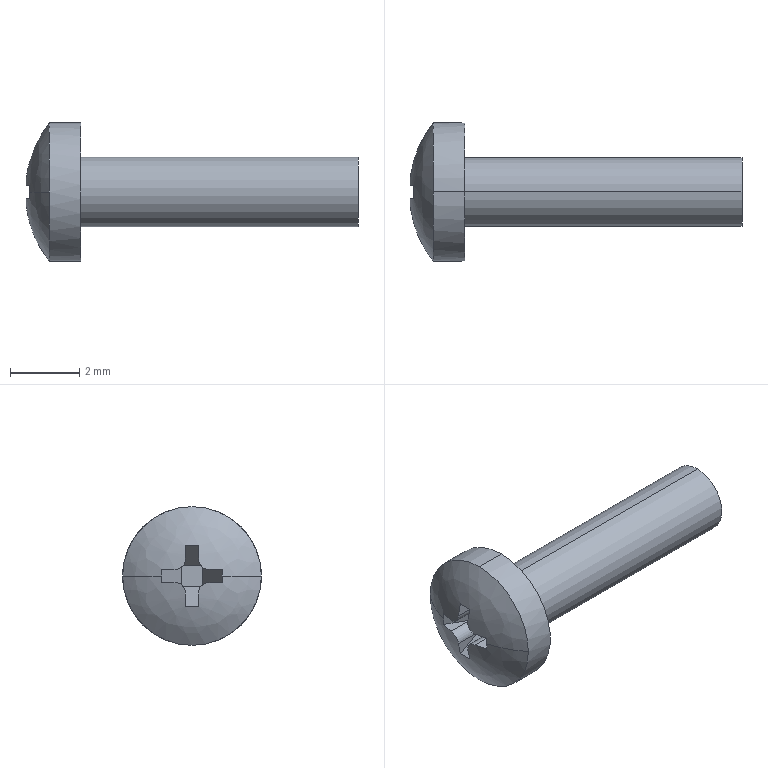Part | SolidWorks | features BaseBody 1 | 1 solid | 25 faces | box 9.576 x 4 x 4 mm | volume 40.085 mm3 | plane 15 | cylinder 8 | spline 2 | commonest cylinder face diameters 0.6 x4 2 x2 4 x2
STEP:
#1=CARTESIAN_POINT('',(0.702,2.,0.));
#2=VERTEX_POINT('',#1);
#3=CARTESIAN_POINT('',(0.702,0.,2.));
#4=VERTEX_POINT('',#3);
#5=CARTESIAN_POINT('',(0.702,0.,0.));
#6=DIRECTION('',(1.,0.,0.));
#7=DIRECTION('',(0.,0.,-1.));
#8=AXIS2_PLACEMENT_3D('',#5,#6,#7);
#9=CIRCLE('',#8,2.);
#10=EDGE_CURVE('',#2,#4,#9,.T.);
#11=ORIENTED_EDGE('',*,*,#10,.F.);
#12=CARTESIAN_POINT('',(0.1231,0.8789,0.));
#13=VERTEX_POINT('',#12);
#14=CARTESIAN_POINT('',(3.2,0.,0.));
#15=DIRECTION('',(0.,0.,1.));
#16=DIRECTION('',(0.,1.,0.));
#17=AXIS2_PLACEMENT_3D('',#14,#15,#16);
#18=CIRCLE('',#17,3.2);
#19=EDGE_CURVE('',#2,#13,#18,.T.);
#20=ORIENTED_EDGE('',*,*,#19,.T.);
#21=CARTESIAN_POINT('',(0.1281,0.876,0.19));
#22=VERTEX_POINT('',#21);
#23=CARTESIAN_POINT('',(0.1231,0.8789,0.));
#24=CARTESIAN_POINT('',(0.1231,0.8789,0.06339));
#25=CARTESIAN_POINT('',(0.1248,0.878,0.1267));
#26=CARTESIAN_POINT('',(0.1281,0.876,0.19));
#27=B_SPLINE_CURVE_WITH_KNOTS('',3,(#23,#24,#25,#26),.UNSPECIFIED.,.F.,.F.,(4,4),(0.,1.),.UNSPECIFIED.);
#28=EDGE_CURVE('',#13,#22,#27,.T.);
#29=ORIENTED_EDGE('',*,*,#28,.T.);
#30=CARTESIAN_POINT('',(0.04345,0.49,0.19));
#31=VERTEX_POINT('',#30);
#32=CARTESIAN_POINT('',(0.1281,0.876,0.19));
#33=CARTESIAN_POINT('',(0.09192,0.7491,0.19));
#34=CARTESIAN_POINT('',(0.0637,0.6204,0.19));
#35=CARTESIAN_POINT('',(0.04345,0.49,0.19));
#36=B_SPLINE_CURVE_WITH_KNOTS('',3,(#32,#33,#34,#35),.UNSPECIFIED.,.F.,.F.,(4,4),(0.,0.0003952),.UNSPECIFIED.);
#37=EDGE_CURVE('',#22,#31,#36,.T.);
#38=ORIENTED_EDGE('',*,*,#37,.T.);
#39=CARTESIAN_POINT('',(0.04345,0.19,0.49));
#40=VERTEX_POINT('',#39);
#41=CARTESIAN_POINT('',(0.04345,0.49,0.19));
#42=CARTESIAN_POINT('',(0.03125,0.4114,0.19));
#43=CARTESIAN_POINT('',(0.02423,0.3335,0.2223));
#44=CARTESIAN_POINT('',(0.02421,0.2224,0.3333));
#45=CARTESIAN_POINT('',(0.03125,0.19,0.4114));
#46=CARTESIAN_POINT('',(0.04345,0.19,0.49));
#47=B_SPLINE_CURVE_WITH_KNOTS('',3,(#41,#42,#43,#44,#45,#46),.UNSPECIFIED.,.F.,.F.,(4,2,4),(0.,0.0002354,0.0004707),.UNSPECIFIED.);
#48=EDGE_CURVE('',#31,#40,#47,.T.);
#49=ORIENTED_EDGE('',*,*,#48,.T.);
#50=CARTESIAN_POINT('',(0.1281,0.19,0.876));
#51=VERTEX_POINT('',#50);
#52=CARTESIAN_POINT('',(3.2,0.19,0.));
#53=DIRECTION('',(0.,1.,0.));
#54=DIRECTION('',(0.,0.,1.));
#55=AXIS2_PLACEMENT_3D('',#52,#53,#54);
#56=CIRCLE('',#55,3.194);
#57=EDGE_CURVE('',#40,#51,#56,.T.);
#58=ORIENTED_EDGE('',*,*,#57,.T.);
#59=CARTESIAN_POINT('',(0.1281,-0.19,0.876));
#60=VERTEX_POINT('',#59);
#61=CARTESIAN_POINT('',(0.1281,0.19,0.876));
#62=CARTESIAN_POINT('',(0.1214,0.06333,0.8799));
#63=CARTESIAN_POINT('',(0.1214,-0.06333,0.8799));
#64=CARTESIAN_POINT('',(0.1281,-0.19,0.876));
#65=B_SPLINE_CURVE_WITH_KNOTS('',3,(#61,#62,#63,#64),.UNSPECIFIED.,.F.,.F.,(4,4),(0.,0.00038),.UNSPECIFIED.);
#66=EDGE_CURVE('',#51,#60,#65,.T.);
#67=ORIENTED_EDGE('',*,*,#66,.T.);
#68=CARTESIAN_POINT('',(0.04345,-0.19,0.49));
#69=VERTEX_POINT('',#68);
#70=CARTESIAN_POINT('',(3.2,-0.19,0.));
#71=DIRECTION('',(0.,-1.,0.));
#72=DIRECTION('',(0.,0.,1.));
#73=AXIS2_PLACEMENT_3D('',#70,#71,#72);
#74=CIRCLE('',#73,3.194);
#75=EDGE_CURVE('',#60,#69,#74,.T.);
#76=ORIENTED_EDGE('',*,*,#75,.T.);
#77=CARTESIAN_POINT('',(0.04345,-0.49,0.19));
#78=VERTEX_POINT('',#77);
#79=CARTESIAN_POINT('',(0.04345,-0.19,0.49));
#80=CARTESIAN_POINT('',(0.03125,-0.19,0.4114));
#81=CARTESIAN_POINT('',(0.02423,-0.2223,0.3335));
#82=CARTESIAN_POINT('',(0.02421,-0.3333,0.2224));
#83=CARTESIAN_POINT('',(0.03125,-0.4114,0.19));
#84=CARTESIAN_POINT('',(0.04345,-0.49,0.19));
#85=B_SPLINE_CURVE_WITH_KNOTS('',3,(#79,#80,#81,#82,#83,#84),.UNSPECIFIED.,.F.,.F.,(4,2,4),(0.,0.0002354,0.0004707),.UNSPECIFIED.);
#86=EDGE_CURVE('',#69,#78,#85,.T.);
#87=ORIENTED_EDGE('',*,*,#86,.T.);
#88=CARTESIAN_POINT('',(0.1281,-0.876,0.19));
#89=VERTEX_POINT('',#88);
#90=CARTESIAN_POINT('',(0.04345,-0.49,0.19));
#91=CARTESIAN_POINT('',(0.0637,-0.6204,0.19));
#92=CARTESIAN_POINT('',(0.09192,-0.7491,0.19));
#93=CARTESIAN_POINT('',(0.1281,-0.876,0.19));
#94=B_SPLINE_CURVE_WITH_KNOTS('',3,(#90,#91,#92,#93),.UNSPECIFIED.,.F.,.F.,(4,4),(0.,0.0003952),.UNSPECIFIED.);
#95=EDGE_CURVE('',#78,#89,#94,.T.);
#96=ORIENTED_EDGE('',*,*,#95,.T.);
#97=CARTESIAN_POINT('',(0.1231,-0.8789,0.));
#98=VERTEX_POINT('',#97);
#99=CARTESIAN_POINT('',(0.1281,-0.876,0.19));
#100=CARTESIAN_POINT('',(0.1248,-0.878,0.1267));
#101=CARTESIAN_POINT('',(0.1231,-0.8789,0.06339));
#102=CARTESIAN_POINT('',(0.1231,-0.8789,0.));
#103=B_SPLINE_CURVE_WITH_KNOTS('',3,(#99,#100,#101,#102),.UNSPECIFIED.,.F.,.F.,(4,4),(0.,1.),.UNSPECIFIED.);
#104=EDGE_CURVE('',#89,#98,#103,.T.);
#105=ORIENTED_EDGE('',*,*,#104,.T.);
#106=CARTESIAN_POINT('',(0.702,-2.,0.));
#107=VERTEX_POINT('',#106);
#108=CARTESIAN_POINT('',(3.2,0.,0.));
#109=DIRECTION('',(0.,0.,1.));
#110=DIRECTION('',(0.,1.,0.));
#111=AXIS2_PLACEMENT_3D('',#108,#109,#110);
#112=CIRCLE('',#111,3.2);
#113=EDGE_CURVE('',#98,#107,#112,.T.);
#114=ORIENTED_EDGE('',*,*,#113,.T.);
#115=CARTESIAN_POINT('',(0.702,0.,0.));
#116=DIRECTION('',(1.,0.,0.));
#117=DIRECTION('',(0.,0.,-1.));
#118=AXIS2_PLACEMENT_3D('',#115,#116,#117);
#119=CIRCLE('',#118,2.);
#120=EDGE_CURVE('',#4,#107,#119,.T.);
#121=ORIENTED_EDGE('',*,*,#120,.F.);
#122=EDGE_LOOP('',(#11,#20,#29,#38,#49,#58,#67,#76,#87,#96,#105,#114,#121));
#123=FACE_OUTER_BOUND('',#122,.T.);
#124=CARTESIAN_POINT('',(0.7183,2.02,0.));
#125=CARTESIAN_POINT('',(0.7183,2.02,0.5729));
#126=CARTESIAN_POINT('',(0.9091,2.02,1.113));
#127=CARTESIAN_POINT('',(1.269,2.02,1.559));
#128=CARTESIAN_POINT('',(-0.2816,0.7919,0.));
#129=CARTESIAN_POINT('',(-0.2816,0.7919,0.8037));
#130=CARTESIAN_POINT('',(-0.01383,0.7919,1.562));
#131=CARTESIAN_POINT('',(0.491,0.7919,2.187));
#132=CARTESIAN_POINT('',(-0.2816,-0.7919,0.));
#133=CARTESIAN_POINT('',(-0.2816,-0.7919,0.8037));
#134=CARTESIAN_POINT('',(-0.01383,-0.7919,1.562));
#135=CARTESIAN_POINT('',(0.491,-0.7919,2.187));
#136=CARTESIAN_POINT('',(0.7183,-2.02,0.));
#137=CARTESIAN_POINT('',(0.7183,-2.02,0.5729));
#138=CARTESIAN_POINT('',(0.9091,-2.02,1.113));
#139=CARTESIAN_POINT('',(1.269,-2.02,1.559));
#140=(BOUNDED_SURFACE()B_SPLINE_SURFACE(3,3,((#124,#125,#126,#127),(#128,#129,#130,#131),(#132,#133,#134,#135),(#136,#137,#138,#139)),.UNSPECIFIED.,.F.,.F.,.F.)B_SPLINE_SURFACE_WITH_KNOTS((4,4),(4,4),(0.,1.),(0.,1.),.UNSPECIFIED.)GEOMETRIC_REPRESENTATION_ITEM()RATIONAL_B_SPLINE_SURFACE(((1.,0.9619,0.9619,1.),(0.8504,0.818,0.818,0.8504),(0.8504,0.818,0.818,0.8504),(1.,0.9619,0.9619,1.)))REPRESENTATION_ITEM('')SURFACE());
#141=ADVANCED_FACE('',(#123),#140,.T.);
#142=CARTESIAN_POINT('',(1.6,0.,-1.));
#143=VERTEX_POINT('',#142);
#144=CARTESIAN_POINT('',(1.6,0.,1.));
#145=VERTEX_POINT('',#144);
#146=CARTESIAN_POINT('',(1.6,0.,0.));
#147=DIRECTION('',(1.,0.,0.));
#148=DIRECTION('',(0.,0.,-1.));
#149=AXIS2_PLACEMENT_3D('',#146,#147,#148);
#150=CIRCLE('',#149,1.);
#151=EDGE_CURVE('',#143,#145,#150,.T.);
#152=ORIENTED_EDGE('',*,*,#151,.T.);
#153=CARTESIAN_POINT('',(9.6,0.,1.));
#154=VERTEX_POINT('',#153);
#155=CARTESIAN_POINT('',(4.516,0.,1.));
#156=DIRECTION('',(1.,0.,0.));
#157=VECTOR('',#156,1000.);
#158=LINE('',#155,#157);
#159=EDGE_CURVE('',#145,#154,#158,.T.);
#160=ORIENTED_EDGE('',*,*,#159,.T.);
#161=CARTESIAN_POINT('',(9.6,0.,-1.));
#162=VERTEX_POINT('',#161);
#163=CARTESIAN_POINT('',(9.6,0.,0.));
#164=DIRECTION('',(-1.,0.,0.));
#165=DIRECTION('',(0.,0.,-1.));
#166=AXIS2_PLACEMENT_3D('',#163,#164,#165);
#167=CIRCLE('',#166,1.);
#168=EDGE_CURVE('',#154,#162,#167,.T.);
#169=ORIENTED_EDGE('',*,*,#168,.T.);
#170=CARTESIAN_POINT('',(4.516,0.,-1.));
#171=DIRECTION('',(1.,0.,0.));
#172=VECTOR('',#171,1000.);
#173=LINE('',#170,#172);
#174=EDGE_CURVE('',#143,#162,#173,.T.);
#175=ORIENTED_EDGE('',*,*,#174,.F.);
#176=EDGE_LOOP('',(#152,#160,#169,#175));
#177=FACE_OUTER_BOUND('',#176,.T.);
#178=CARTESIAN_POINT('',(4.516,0.,0.));
#179=DIRECTION('',(1.,0.,0.));
#180=DIRECTION('',(0.,0.,-1.));
#181=AXIS2_PLACEMENT_3D('',#178,#179,#180);
#182=CYLINDRICAL_SURFACE('',#181,1.);
#183=ADVANCED_FACE('',(#177),#182,.T.);
#184=CARTESIAN_POINT('',(0.702,0.,-2.));
#185=VERTEX_POINT('',#184);
#186=CARTESIAN_POINT('',(0.702,0.,0.));
#187=DIRECTION('',(1.,0.,0.));
#188=DIRECTION('',(0.,0.,-1.));
#189=AXIS2_PLACEMENT_3D('',#186,#187,#188);
#190=CIRCLE('',#189,2.);
#191=EDGE_CURVE('',#185,#2,#190,.T.);
#192=ORIENTED_EDGE('',*,*,#191,.T.);
#193=ORIENTED_EDGE('',*,*,#10,.T.);
#194=CARTESIAN_POINT('',(1.6,0.,2.));
#195=VERTEX_POINT('',#194);
#196=CARTESIAN_POINT('',(4.516,0.,2.));
#197=DIRECTION('',(1.,0.,0.));
#198=VECTOR('',#197,1000.);
#199=LINE('',#196,#198);
#200=EDGE_CURVE('',#4,#195,#199,.T.);
#201=ORIENTED_EDGE('',*,*,#200,.T.);
#202=CARTESIAN_POINT('',(1.6,0.,-2.));
#203=VERTEX_POINT('',#202);
#204=CARTESIAN_POINT('',(1.6,0.,0.));
#205=DIRECTION('',(1.,0.,0.));
#206=DIRECTION('',(0.,0.,-1.));
#207=AXIS2_PLACEMENT_3D('',#204,#205,#206);
#208=CIRCLE('',#207,2.);
#209=EDGE_CURVE('',#203,#195,#208,.T.);
#210=ORIENTED_EDGE('',*,*,#209,.F.);
#211=CARTESIAN_POINT('',(4.516,0.,-2.));
#212=DIRECTION('',(1.,0.,0.));
#213=VECTOR('',#212,1000.);
#214=LINE('',#211,#213);
#215=EDGE_CURVE('',#185,#203,#214,.T.);
#216=ORIENTED_EDGE('',*,*,#215,.F.);
#217=EDGE_LOOP('',(#192,#193,#201,#210,#216));
#218=FACE_OUTER_BOUND('',#217,.T.);
#219=CARTESIAN_POINT('',(4.516,0.,0.));
#220=DIRECTION('',(1.,0.,0.));
#221=DIRECTION('',(0.,0.,-1.));
#222=AXIS2_PLACEMENT_3D('',#219,#220,#221);
#223=CYLINDRICAL_SURFACE('',#222,2.);
#224=ADVANCED_FACE('',(#218),#223,.T.);
#225=ORIENTED_EDGE('',*,*,#159,.F.);
#226=CARTESIAN_POINT('',(1.6,0.,0.));
#227=DIRECTION('',(1.,0.,0.));
#228=DIRECTION('',(0.,0.,-1.));
#229=AXIS2_PLACEMENT_3D('',#226,#227,#228);
#230=CIRCLE('',#229,1.);
#231=EDGE_CURVE('',#145,#143,#230,.T.);
#232=ORIENTED_EDGE('',*,*,#231,.T.);
#233=ORIENTED_EDGE('',*,*,#174,.T.);
#234=CARTESIAN_POINT('',(9.6,0.,0.));
#235=DIRECTION('',(-1.,0.,0.));
#236=DIRECTION('',(0.,0.,-1.));
#237=AXIS2_PLACEMENT_3D('',#234,#235,#236);
#238=CIRCLE('',#237,1.);
#239=EDGE_CURVE('',#162,#154,#238,.T.);
#240=ORIENTED_EDGE('',*,*,#239,.T.);
#241=EDGE_LOOP('',(#225,#232,#233,#240));
#242=FACE_OUTER_BOUND('',#241,.T.);
#243=CARTESIAN_POINT('',(4.516,0.,0.));
#244=DIRECTION('',(1.,0.,0.));
#245=DIRECTION('',(0.,0.,-1.));
#246=AXIS2_PLACEMENT_3D('',#243,#244,#245);
#247=CYLINDRICAL_SURFACE('',#246,1.);
#248=ADVANCED_FACE('',(#242),#247,.T.);
#249=ORIENTED_EDGE('',*,*,#239,.F.);
#250=ORIENTED_EDGE('',*,*,#168,.F.);
#251=EDGE_LOOP('',(#249,#250));
#252=FACE_OUTER_BOUND('',#251,.T.);
#253=CARTESIAN_POINT('',(9.6,1.,0.));
#254=DIRECTION('',(1.,0.,0.));
#255=DIRECTION('',(0.,0.,-1.));
#256=AXIS2_PLACEMENT_3D('',#253,#254,#255);
#257=PLANE('',#256);
#258=ADVANCED_FACE('',(#252),#257,.T.);
#259=ORIENTED_EDGE('',*,*,#151,.F.);
#260=ORIENTED_EDGE('',*,*,#231,.F.);
#261=EDGE_LOOP('',(#259,#260));
#262=FACE_BOUND('',#261,.T.);
#263=ORIENTED_EDGE('',*,*,#209,.T.);
#264=CARTESIAN_POINT('',(1.6,0.,0.));
#265=DIRECTION('',(1.,0.,0.));
#266=DIRECTION('',(0.,0.,-1.));
#267=AXIS2_PLACEMENT_3D('',#264,#265,#266);
#268=CIRCLE('',#267,2.);
#269=EDGE_CURVE('',#195,#203,#268,.T.);
#270=ORIENTED_EDGE('',*,*,#269,.T.);
#271=EDGE_LOOP('',(#263,#270));
#272=FACE_OUTER_BOUND('',#271,.T.);
#273=CARTESIAN_POINT('',(1.6,1.3,0.));
#274=DIRECTION('',(1.,0.,0.));
#275=DIRECTION('',(0.,0.,-1.));
#276=AXIS2_PLACEMENT_3D('',#273,#274,#275);
#277=PLANE('',#276);
#278=ADVANCED_FACE('',(#262,#272),#277,.T.);
#279=ORIENTED_EDGE('',*,*,#200,.F.);
#280=ORIENTED_EDGE('',*,*,#120,.T.);
#281=CARTESIAN_POINT('',(0.702,0.,0.));
#282=DIRECTION('',(1.,0.,0.));
#283=DIRECTION('',(0.,0.,-1.));
#284=AXIS2_PLACEMENT_3D('',#281,#282,#283);
#285=CIRCLE('',#284,2.);
#286=EDGE_CURVE('',#107,#185,#285,.T.);
#287=ORIENTED_EDGE('',*,*,#286,.T.);
#288=ORIENTED_EDGE('',*,*,#215,.T.);
#289=ORIENTED_EDGE('',*,*,#269,.F.);
#290=EDGE_LOOP('',(#279,#280,#287,#288,#289));
#291=FACE_OUTER_BOUND('',#290,.T.);
#292=CARTESIAN_POINT('',(4.516,0.,0.));
#293=DIRECTION('',(1.,0.,0.));
#294=DIRECTION('',(0.,0.,-1.));
#295=AXIS2_PLACEMENT_3D('',#292,#293,#294);
#296=CYLINDRICAL_SURFACE('',#295,2.);
#297=ADVANCED_FACE('',(#291),#296,.T.);
#298=ORIENTED_EDGE('',*,*,#19,.F.);
#299=ORIENTED_EDGE('',*,*,#191,.F.);
#300=ORIENTED_EDGE('',*,*,#286,.F.);
#301=ORIENTED_EDGE('',*,*,#113,.F.);
#302=CARTESIAN_POINT('',(0.1281,-0.876,-0.19));
#303=VERTEX_POINT('',#302);
#304=CARTESIAN_POINT('',(0.1231,-0.8789,0.));
#305=CARTESIAN_POINT('',(0.1231,-0.8789,-0.06339));
#306=CARTESIAN_POINT('',(0.1248,-0.878,-0.1267));
#307=CARTESIAN_POINT('',(0.1281,-0.876,-0.19));
#308=B_SPLINE_CURVE_WITH_KNOTS('',3,(#304,#305,#306,#307),.UNSPECIFIED.,.F.,.F.,(4,4),(0.,1.),.UNSPECIFIED.);
#309=EDGE_CURVE('',#98,#303,#308,.T.);
#310=ORIENTED_EDGE('',*,*,#309,.T.);
#311=CARTESIAN_POINT('',(0.04345,-0.49,-0.19));
#312=VERTEX_POINT('',#311);
#313=CARTESIAN_POINT('',(0.1281,-0.876,-0.19));
#314=CARTESIAN_POINT('',(0.09192,-0.7491,-0.19));
#315=CARTESIAN_POINT('',(0.0637,-0.6204,-0.19));
#316=CARTESIAN_POINT('',(0.04345,-0.49,-0.19));
#317=B_SPLINE_CURVE_WITH_KNOTS('',3,(#313,#314,#315,#316),.UNSPECIFIED.,.F.,.F.,(4,4),(0.,0.0003952),.UNSPECIFIED.);
#318=EDGE_CURVE('',#303,#312,#317,.T.);
#319=ORIENTED_EDGE('',*,*,#318,.T.);
#320=CARTESIAN_POINT('',(0.04345,-0.19,-0.49));
#321=VERTEX_POINT('',#320);
#322=CARTESIAN_POINT('',(0.04345,-0.49,-0.19));
#323=CARTESIAN_POINT('',(0.03125,-0.4114,-0.19));
#324=CARTESIAN_POINT('',(0.02423,-0.3335,-0.2223));
#325=CARTESIAN_POINT('',(0.02421,-0.2224,-0.3333));
#326=CARTESIAN_POINT('',(0.03125,-0.19,-0.4114));
#327=CARTESIAN_POINT('',(0.04345,-0.19,-0.49));
#328=B_SPLINE_CURVE_WITH_KNOTS('',3,(#322,#323,#324,#325,#326,#327),.UNSPECIFIED.,.F.,.F.,(4,2,4),(0.,0.0002354,0.0004707),.UNSPECIFIED.);
#329=EDGE_CURVE('',#312,#321,#328,.T.);
#330=ORIENTED_EDGE('',*,*,#329,.T.);
#331=CARTESIAN_POINT('',(0.1281,-0.19,-0.876));
#332=VERTEX_POINT('',#331);
#333=CARTESIAN_POINT('',(3.2,-0.19,0.));
#334=DIRECTION('',(0.,-1.,0.));
#335=DIRECTION('',(0.,0.,1.));
#336=AXIS2_PLACEMENT_3D('',#333,#334,#335);
#337=CIRCLE('',#336,3.194);
#338=EDGE_CURVE('',#321,#332,#337,.T.);
#339=ORIENTED_EDGE('',*,*,#338,.T.);
#340=CARTESIAN_POINT('',(0.1281,0.19,-0.876));
#341=VERTEX_POINT('',#340);
#342=CARTESIAN_POINT('',(0.1281,-0.19,-0.876));
#343=CARTESIAN_POINT('',(0.1214,-0.06333,-0.8799));
#344=CARTESIAN_POINT('',(0.1214,0.06333,-0.8799));
#345=CARTESIAN_POINT('',(0.1281,0.19,-0.876));
#346=B_SPLINE_CURVE_WITH_KNOTS('',3,(#342,#343,#344,#345),.UNSPECIFIED.,.F.,.F.,(4,4),(0.,0.00038),.UNSPECIFIED.);
#347=EDGE_CURVE('',#332,#341,#346,.T.);
#348=ORIENTED_EDGE('',*,*,#347,.T.);
#349=CARTESIAN_POINT('',(0.04345,0.19,-0.49));
#350=VERTEX_POINT('',#349);
#351=CARTESIAN_POINT('',(3.2,0.19,0.));
#352=DIRECTION('',(0.,1.,0.));
#353=DIRECTION('',(0.,0.,1.));
#354=AXIS2_PLACEMENT_3D('',#351,#352,#353);
#355=CIRCLE('',#354,3.194);
#356=EDGE_CURVE('',#341,#350,#355,.T.);
#357=ORIENTED_EDGE('',*,*,#356,.T.);
#358=CARTESIAN_POINT('',(0.04345,0.49,-0.19));
#359=VERTEX_POINT('',#358);
#360=CARTESIAN_POINT('',(0.04345,0.19,-0.49));
#361=CARTESIAN_POINT('',(0.03125,0.19,-0.4114));
#362=CARTESIAN_POINT('',(0.02423,0.2223,-0.3335));
#363=CARTESIAN_POINT('',(0.02421,0.3333,-0.2224));
#364=CARTESIAN_POINT('',(0.03125,0.4114,-0.19));
#365=CARTESIAN_POINT('',(0.04345,0.49,-0.19));
#366=B_SPLINE_CURVE_WITH_KNOTS('',3,(#360,#361,#362,#363,#364,#365),.UNSPECIFIED.,.F.,.F.,(4,2,4),(0.,0.0002354,0.0004707),.UNSPECIFIED.);
#367=EDGE_CURVE('',#350,#359,#366,.T.);
#368=ORIENTED_EDGE('',*,*,#367,.T.);
#369=CARTESIAN_POINT('',(0.1281,0.876,-0.19));
#370=VERTEX_POINT('',#369);
#371=CARTESIAN_POINT('',(0.04345,0.49,-0.19));
#372=CARTESIAN_POINT('',(0.0637,0.6204,-0.19));
#373=CARTESIAN_POINT('',(0.09192,0.7491,-0.19));
#374=CARTESIAN_POINT('',(0.1281,0.876,-0.19));
#375=B_SPLINE_CURVE_WITH_KNOTS('',3,(#371,#372,#373,#374),.UNSPECIFIED.,.F.,.F.,(4,4),(0.,0.0003952),.UNSPECIFIED.);
#376=EDGE_CURVE('',#359,#370,#375,.T.);
#377=ORIENTED_EDGE('',*,*,#376,.T.);
#378=CARTESIAN_POINT('',(0.1281,0.876,-0.19));
#379=CARTESIAN_POINT('',(0.1248,0.878,-0.1267));
#380=CARTESIAN_POINT('',(0.1231,0.8789,-0.06339));
#381=CARTESIAN_POINT('',(0.1231,0.8789,0.));
#382=B_SPLINE_CURVE_WITH_KNOTS('',3,(#378,#379,#380,#381),.UNSPECIFIED.,.F.,.F.,(4,4),(0.,1.),.UNSPECIFIED.);
#383=EDGE_CURVE('',#370,#13,#382,.T.);
#384=ORIENTED_EDGE('',*,*,#383,.T.);
#385=EDGE_LOOP('',(#298,#299,#300,#301,#310,#319,#330,#339,#348,#357,#368,#377,#384));
#386=FACE_OUTER_BOUND('',#385,.T.);
#387=CARTESIAN_POINT('',(1.269,2.02,-1.559));
#388=CARTESIAN_POINT('',(0.9091,2.02,-1.113));
#389=CARTESIAN_POINT('',(0.7183,2.02,-0.5729));
#390=CARTESIAN_POINT('',(0.7183,2.02,0.));
#391=CARTESIAN_POINT('',(0.491,0.7919,-2.187));
#392=CARTESIAN_POINT('',(-0.01383,0.7919,-1.562));
#393=CARTESIAN_POINT('',(-0.2816,0.7919,-0.8037));
#394=CARTESIAN_POINT('',(-0.2816,0.7919,0.));
#395=CARTESIAN_POINT('',(0.491,-0.7919,-2.187));
#396=CARTESIAN_POINT('',(-0.01383,-0.7919,-1.562));
#397=CARTESIAN_POINT('',(-0.2816,-0.7919,-0.8037));
#398=CARTESIAN_POINT('',(-0.2816,-0.7919,0.));
#399=CARTESIAN_POINT('',(1.269,-2.02,-1.559));
#400=CARTESIAN_POINT('',(0.9091,-2.02,-1.113));
#401=CARTESIAN_POINT('',(0.7183,-2.02,-0.5729));
#402=CARTESIAN_POINT('',(0.7183,-2.02,0.));
#403=(BOUNDED_SURFACE()B_SPLINE_SURFACE(3,3,((#387,#388,#389,#390),(#391,#392,#393,#394),(#395,#396,#397,#398),(#399,#400,#401,#402)),.UNSPECIFIED.,.F.,.F.,.F.)B_SPLINE_SURFACE_WITH_KNOTS((4,4),(4,4),(0.,1.),(0.,1.),.UNSPECIFIED.)GEOMETRIC_REPRESENTATION_ITEM()RATIONAL_B_SPLINE_SURFACE(((1.,0.9619,0.9619,1.),(0.8504,0.818,0.818,0.8504),(0.8504,0.818,0.818,0.8504),(1.,0.9619,0.9619,1.)))REPRESENTATION_ITEM('')SURFACE());
#404=ADVANCED_FACE('',(#386),#403,.T.);
#405=ORIENTED_EDGE('',*,*,#28,.F.);
#406=ORIENTED_EDGE('',*,*,#383,.F.);
#407=CARTESIAN_POINT('',(0.7967,0.49,-0.19));
#408=VERTEX_POINT('',#407);
#409=CARTESIAN_POINT('',(0.,0.95,-0.19));
#410=DIRECTION('',(0.866,-0.5,0.));
#411=VECTOR('',#410,1000.);
#412=LINE('',#409,#411);
#413=EDGE_CURVE('',#370,#408,#412,.T.);
#414=ORIENTED_EDGE('',*,*,#413,.T.);
#415=CARTESIAN_POINT('',(1.12,0.3034,-0.2551));
#416=VERTEX_POINT('',#415);
#417=CARTESIAN_POINT('',(0.7967,0.49,-0.19));
#418=CARTESIAN_POINT('',(0.9153,0.4216,-0.19));
#419=CARTESIAN_POINT('',(1.027,0.3569,-0.2125));
#420=CARTESIAN_POINT('',(1.12,0.3034,-0.2551));
#421=(BOUNDED_CURVE()B_SPLINE_CURVE(3,(#417,#418,#419,#420),.UNSPECIFIED.,.F.,.F.)B_SPLINE_CURVE_WITH_KNOTS((4,4),(1.571,2.242),.UNSPECIFIED.)CURVE()GEOMETRIC_REPRESENTATION_ITEM()RATIONAL_B_SPLINE_CURVE((1.,0.9628,0.9628,1.))REPRESENTATION_ITEM(''));
#422=EDGE_CURVE('',#408,#416,#421,.T.);
#423=ORIENTED_EDGE('',*,*,#422,.T.);
#424=CARTESIAN_POINT('',(1.12,0.3034,0.2551));
#425=VERTEX_POINT('',#424);
#426=CARTESIAN_POINT('',(1.12,0.3034,0.));
#427=DIRECTION('',(0.,0.,1.));
#428=VECTOR('',#427,1000.);
#429=LINE('',#426,#428);
#430=EDGE_CURVE('',#416,#425,#429,.T.);
#431=ORIENTED_EDGE('',*,*,#430,.T.);
#432=CARTESIAN_POINT('',(0.7967,0.49,0.19));
#433=VERTEX_POINT('',#432);
#434=CARTESIAN_POINT('',(1.12,0.3034,0.2551));
#435=CARTESIAN_POINT('',(1.027,0.3569,0.2125));
#436=CARTESIAN_POINT('',(0.9153,0.4216,0.19));
#437=CARTESIAN_POINT('',(0.7967,0.49,0.19));
#438=(BOUNDED_CURVE()B_SPLINE_CURVE(3,(#434,#435,#436,#437),.UNSPECIFIED.,.F.,.F.)B_SPLINE_CURVE_WITH_KNOTS((4,4),(4.041,4.712),.UNSPECIFIED.)CURVE()GEOMETRIC_REPRESENTATION_ITEM()RATIONAL_B_SPLINE_CURVE((1.,0.9628,0.9628,1.))REPRESENTATION_ITEM(''));
#439=EDGE_CURVE('',#425,#433,#438,.T.);
#440=ORIENTED_EDGE('',*,*,#439,.T.);
#441=CARTESIAN_POINT('',(0.,0.95,0.19));
#442=DIRECTION('',(-0.866,0.5,0.));
#443=VECTOR('',#442,1000.);
#444=LINE('',#441,#443);
#445=EDGE_CURVE('',#433,#22,#444,.T.);
#446=ORIENTED_EDGE('',*,*,#445,.T.);
#447=EDGE_LOOP('',(#405,#406,#414,#423,#431,#440,#446));
#448=FACE_OUTER_BOUND('',#447,.T.);
#449=CARTESIAN_POINT('',(0.,0.95,0.));
#450=DIRECTION('',(-0.5,-0.866,0.));
#451=DIRECTION('',(0.866,-0.5,0.));
#452=AXIS2_PLACEMENT_3D('',#449,#450,#451);
#453=PLANE('',#452);
#454=ADVANCED_FACE('',(#448),#453,.T.);
#455=CARTESIAN_POINT('',(1.12,0.49,-0.19));
#456=DIRECTION('',(1.,0.,0.));
#457=VECTOR('',#456,1000.);
#458=LINE('',#455,#457);
#459=EDGE_CURVE('',#359,#408,#458,.T.);
#460=ORIENTED_EDGE('',*,*,#459,.T.);
#461=ORIENTED_EDGE('',*,*,#413,.F.);
#462=ORIENTED_EDGE('',*,*,#376,.F.);
#463=EDGE_LOOP('',(#460,#461,#462));
#464=FACE_OUTER_BOUND('',#463,.T.);
#465=CARTESIAN_POINT('',(1.12,0.19,-0.19));
#466=DIRECTION('',(0.,0.,1.));
#467=DIRECTION('',(1.,0.,0.));
#468=AXIS2_PLACEMENT_3D('',#465,#466,#467);
#469=PLANE('',#468);
#470=ADVANCED_FACE('',(#464),#469,.T.);
#471=CARTESIAN_POINT('',(0.7967,0.19,-0.49));
#472=VERTEX_POINT('',#471);
#473=CARTESIAN_POINT('',(1.12,0.19,-0.49));
#474=DIRECTION('',(1.,0.,0.));
#475=VECTOR('',#474,1000.);
#476=LINE('',#473,#475);
#477=EDGE_CURVE('',#350,#472,#476,.T.);
#478=ORIENTED_EDGE('',*,*,#477,.T.);
#479=CARTESIAN_POINT('',(1.12,0.2551,-0.3034));
#480=VERTEX_POINT('',#479);
#481=CARTESIAN_POINT('',(0.7967,0.19,-0.49));
#482=CARTESIAN_POINT('',(0.9153,0.19,-0.4216));
#483=CARTESIAN_POINT('',(1.027,0.2125,-0.3569));
#484=CARTESIAN_POINT('',(1.12,0.2551,-0.3034));
#485=(BOUNDED_CURVE()B_SPLINE_CURVE(3,(#481,#482,#483,#484),.UNSPECIFIED.,.F.,.F.)B_SPLINE_CURVE_WITH_KNOTS((4,4),(1.571,2.242),.UNSPECIFIED.)CURVE()GEOMETRIC_REPRESENTATION_ITEM()RATIONAL_B_SPLINE_CURVE((1.,0.9628,0.9628,1.))REPRESENTATION_ITEM(''));
#486=EDGE_CURVE('',#472,#480,#485,.T.);
#487=ORIENTED_EDGE('',*,*,#486,.T.);
#488=CARTESIAN_POINT('',(1.12,0.49,-0.49));
#489=DIRECTION('',(-1.,0.,0.));
#490=DIRECTION('',(0.,0.,1.));
#491=AXIS2_PLACEMENT_3D('',#488,#489,#490);
#492=CIRCLE('',#491,0.3);
#493=EDGE_CURVE('',#480,#416,#492,.T.);
#494=ORIENTED_EDGE('',*,*,#493,.T.);
#495=ORIENTED_EDGE('',*,*,#422,.F.);
#496=ORIENTED_EDGE('',*,*,#459,.F.);
#497=ORIENTED_EDGE('',*,*,#367,.F.);
#498=EDGE_LOOP('',(#478,#487,#494,#495,#496,#497));
#499=FACE_OUTER_BOUND('',#498,.T.);
#500=CARTESIAN_POINT('',(1.12,0.49,-0.49));
#501=DIRECTION('',(-1.,0.,0.));
#502=DIRECTION('',(0.,0.,1.));
#503=AXIS2_PLACEMENT_3D('',#500,#501,#502);
#504=CYLINDRICAL_SURFACE('',#503,0.3);
#505=ADVANCED_FACE('',(#499),#504,.T.);
#506=ORIENTED_EDGE('',*,*,#477,.F.);
#507=ORIENTED_EDGE('',*,*,#356,.F.);
#508=CARTESIAN_POINT('',(0.1281,0.19,-0.876));
#509=DIRECTION('',(0.866,0.,0.5));
#510=VECTOR('',#509,1000.);
#511=LINE('',#508,#510);
#512=EDGE_CURVE('',#341,#472,#511,.T.);
#513=ORIENTED_EDGE('',*,*,#512,.T.);
#514=EDGE_LOOP('',(#506,#507,#513));
#515=FACE_OUTER_BOUND('',#514,.T.);
#516=CARTESIAN_POINT('',(1.12,0.19,-0.19));
#517=DIRECTION('',(0.,-1.,0.));
#518=DIRECTION('',(0.,0.,-1.));
#519=AXIS2_PLACEMENT_3D('',#516,#517,#518);
#520=PLANE('',#519);
#521=ADVANCED_FACE('',(#515),#520,.T.);
#522=ORIENTED_EDGE('',*,*,#512,.F.);
#523=ORIENTED_EDGE('',*,*,#347,.F.);
#524=CARTESIAN_POINT('',(0.7967,-0.19,-0.49));
#525=VERTEX_POINT('',#524);
#526=CARTESIAN_POINT('',(0.,-0.19,-0.95));
#527=DIRECTION('',(0.866,0.,0.5));
#528=VECTOR('',#527,1000.);
#529=LINE('',#526,#528);
#530=EDGE_CURVE('',#332,#525,#529,.T.);
#531=ORIENTED_EDGE('',*,*,#530,.T.);
#532=CARTESIAN_POINT('',(1.12,-0.2551,-0.3034));
#533=VERTEX_POINT('',#532);
#534=CARTESIAN_POINT('',(0.7967,-0.19,-0.49));
#535=CARTESIAN_POINT('',(0.9153,-0.19,-0.4216));
#536=CARTESIAN_POINT('',(1.027,-0.2125,-0.3569));
#537=CARTESIAN_POINT('',(1.12,-0.2551,-0.3034));
#538=(BOUNDED_CURVE()B_SPLINE_CURVE(3,(#534,#535,#536,#537),.UNSPECIFIED.,.F.,.F.)B_SPLINE_CURVE_WITH_KNOTS((4,4),(1.571,2.242),.UNSPECIFIED.)CURVE()GEOMETRIC_REPRESENTATION_ITEM()RATIONAL_B_SPLINE_CURVE((1.,0.9628,0.9628,1.))REPRESENTATION_ITEM(''));
#539=EDGE_CURVE('',#525,#533,#538,.T.);
#540=ORIENTED_EDGE('',*,*,#539,.T.);
#541=CARTESIAN_POINT('',(1.12,0.,-0.3034));
#542=DIRECTION('',(0.,1.,0.));
#543=VECTOR('',#542,1000.);
#544=LINE('',#541,#543);
#545=EDGE_CURVE('',#533,#480,#544,.T.);
#546=ORIENTED_EDGE('',*,*,#545,.T.);
#547=ORIENTED_EDGE('',*,*,#486,.F.);
#548=EDGE_LOOP('',(#522,#523,#531,#540,#546,#547));
#549=FACE_OUTER_BOUND('',#548,.T.);
#550=CARTESIAN_POINT('',(0.,0.,-0.95));
#551=DIRECTION('',(-0.5,0.,0.866));
#552=DIRECTION('',(0.866,0.,0.5));
#553=AXIS2_PLACEMENT_3D('',#550,#551,#552);
#554=PLANE('',#553);
#555=ADVANCED_FACE('',(#549),#554,.T.);
#556=CARTESIAN_POINT('',(1.12,-0.19,-0.49));
#557=DIRECTION('',(1.,0.,0.));
#558=VECTOR('',#557,1000.);
#559=LINE('',#556,#558);
#560=EDGE_CURVE('',#321,#525,#559,.T.);
#561=ORIENTED_EDGE('',*,*,#560,.T.);
#562=ORIENTED_EDGE('',*,*,#530,.F.);
#563=ORIENTED_EDGE('',*,*,#338,.F.);
#564=EDGE_LOOP('',(#561,#562,#563));
#565=FACE_OUTER_BOUND('',#564,.T.);
#566=CARTESIAN_POINT('',(1.12,-0.19,-0.19));
#567=DIRECTION('',(0.,1.,0.));
#568=DIRECTION('',(0.,0.,1.));
#569=AXIS2_PLACEMENT_3D('',#566,#567,#568);
#570=PLANE('',#569);
#571=ADVANCED_FACE('',(#565),#570,.T.);
#572=CARTESIAN_POINT('',(0.7967,-0.49,-0.19));
#573=VERTEX_POINT('',#572);
#574=CARTESIAN_POINT('',(1.12,-0.49,-0.19));
#575=DIRECTION('',(1.,0.,0.));
#576=VECTOR('',#575,1000.);
#577=LINE('',#574,#576);
#578=EDGE_CURVE('',#312,#573,#577,.T.);
#579=ORIENTED_EDGE('',*,*,#578,.T.);
#580=CARTESIAN_POINT('',(1.12,-0.3034,-0.2551));
#581=VERTEX_POINT('',#580);
#582=CARTESIAN_POINT('',(0.7967,-0.49,-0.19));
#583=CARTESIAN_POINT('',(0.9153,-0.4216,-0.19));
#584=CARTESIAN_POINT('',(1.027,-0.3569,-0.2125));
#585=CARTESIAN_POINT('',(1.12,-0.3034,-0.2551));
#586=(BOUNDED_CURVE()B_SPLINE_CURVE(3,(#582,#583,#584,#585),.UNSPECIFIED.,.F.,.F.)B_SPLINE_CURVE_WITH_KNOTS((4,4),(1.571,2.242),.UNSPECIFIED.)CURVE()GEOMETRIC_REPRESENTATION_ITEM()RATIONAL_B_SPLINE_CURVE((1.,0.9628,0.9628,1.))REPRESENTATION_ITEM(''));
#587=EDGE_CURVE('',#573,#581,#586,.T.);
#588=ORIENTED_EDGE('',*,*,#587,.T.);
#589=CARTESIAN_POINT('',(1.12,-0.49,-0.49));
#590=DIRECTION('',(-1.,0.,0.));
#591=DIRECTION('',(0.,0.,1.));
#592=AXIS2_PLACEMENT_3D('',#589,#590,#591);
#593=CIRCLE('',#592,0.3);
#594=EDGE_CURVE('',#581,#533,#593,.T.);
#595=ORIENTED_EDGE('',*,*,#594,.T.);
#596=ORIENTED_EDGE('',*,*,#539,.F.);
#597=ORIENTED_EDGE('',*,*,#560,.F.);
#598=ORIENTED_EDGE('',*,*,#329,.F.);
#599=EDGE_LOOP('',(#579,#588,#595,#596,#597,#598));
#600=FACE_OUTER_BOUND('',#599,.T.);
#601=CARTESIAN_POINT('',(1.12,-0.49,-0.49));
#602=DIRECTION('',(-1.,0.,0.));
#603=DIRECTION('',(0.,0.,1.));
#604=AXIS2_PLACEMENT_3D('',#601,#602,#603);
#605=CYLINDRICAL_SURFACE('',#604,0.3);
#606=ADVANCED_FACE('',(#600),#605,.T.);
#607=ORIENTED_EDGE('',*,*,#578,.F.);
#608=ORIENTED_EDGE('',*,*,#318,.F.);
#609=CARTESIAN_POINT('',(0.1281,-0.876,-0.19));
#610=DIRECTION('',(0.866,0.5,0.));
#611=VECTOR('',#610,1000.);
#612=LINE('',#609,#611);
#613=EDGE_CURVE('',#303,#573,#612,.T.);
#614=ORIENTED_EDGE('',*,*,#613,.T.);
#615=EDGE_LOOP('',(#607,#608,#614));
#616=FACE_OUTER_BOUND('',#615,.T.);
#617=CARTESIAN_POINT('',(1.12,-0.19,-0.19));
#618=DIRECTION('',(0.,0.,1.));
#619=DIRECTION('',(1.,0.,0.));
#620=AXIS2_PLACEMENT_3D('',#617,#618,#619);
#621=PLANE('',#620);
#622=ADVANCED_FACE('',(#616),#621,.T.);
#623=ORIENTED_EDGE('',*,*,#309,.F.);
#624=ORIENTED_EDGE('',*,*,#104,.F.);
#625=CARTESIAN_POINT('',(0.7967,-0.49,0.19));
#626=VERTEX_POINT('',#625);
#627=CARTESIAN_POINT('',(0.,-0.95,0.19));
#628=DIRECTION('',(0.866,0.5,0.));
#629=VECTOR('',#628,1000.);
#630=LINE('',#627,#629);
#631=EDGE_CURVE('',#89,#626,#630,.T.);
#632=ORIENTED_EDGE('',*,*,#631,.T.);
#633=CARTESIAN_POINT('',(1.12,-0.3034,0.2551));
#634=VERTEX_POINT('',#633);
#635=CARTESIAN_POINT('',(0.7967,-0.49,0.19));
#636=CARTESIAN_POINT('',(0.9153,-0.4216,0.19));
#637=CARTESIAN_POINT('',(1.027,-0.3569,0.2125));
#638=CARTESIAN_POINT('',(1.12,-0.3034,0.2551));
#639=(BOUNDED_CURVE()B_SPLINE_CURVE(3,(#635,#636,#637,#638),.UNSPECIFIED.,.F.,.F.)B_SPLINE_CURVE_WITH_KNOTS((4,4),(1.571,2.242),.UNSPECIFIED.)CURVE()GEOMETRIC_REPRESENTATION_ITEM()RATIONAL_B_SPLINE_CURVE((1.,0.9628,0.9628,1.))REPRESENTATION_ITEM(''));
#640=EDGE_CURVE('',#626,#634,#639,.T.);
#641=ORIENTED_EDGE('',*,*,#640,.T.);
#642=CARTESIAN_POINT('',(1.12,-0.3034,0.));
#643=DIRECTION('',(0.,0.,-1.));
#644=VECTOR('',#643,1000.);
#645=LINE('',#642,#644);
#646=EDGE_CURVE('',#634,#581,#645,.T.);
#647=ORIENTED_EDGE('',*,*,#646,.T.);
#648=ORIENTED_EDGE('',*,*,#587,.F.);
#649=ORIENTED_EDGE('',*,*,#613,.F.);
#650=EDGE_LOOP('',(#623,#624,#632,#641,#647,#648,#649));
#651=FACE_OUTER_BOUND('',#650,.T.);
#652=CARTESIAN_POINT('',(0.,-0.95,0.));
#653=DIRECTION('',(-0.5,0.866,0.));
#654=DIRECTION('',(-0.866,-0.5,0.));
#655=AXIS2_PLACEMENT_3D('',#652,#653,#654);
#656=PLANE('',#655);
#657=ADVANCED_FACE('',(#651),#656,.T.);
#658=CARTESIAN_POINT('',(1.12,-0.49,0.19));
#659=DIRECTION('',(1.,0.,0.));
#660=VECTOR('',#659,1000.);
#661=LINE('',#658,#660);
#662=EDGE_CURVE('',#78,#626,#661,.T.);
#663=ORIENTED_EDGE('',*,*,#662,.T.);
#664=ORIENTED_EDGE('',*,*,#631,.F.);
#665=ORIENTED_EDGE('',*,*,#95,.F.);
#666=EDGE_LOOP('',(#663,#664,#665));
#667=FACE_OUTER_BOUND('',#666,.T.);
#668=CARTESIAN_POINT('',(1.12,-0.19,0.19));
#669=DIRECTION('',(0.,0.,-1.));
#670=DIRECTION('',(0.,1.,0.));
#671=AXIS2_PLACEMENT_3D('',#668,#669,#670);
#672=PLANE('',#671);
#673=ADVANCED_FACE('',(#667),#672,.T.);
#674=CARTESIAN_POINT('',(0.7967,-0.19,0.49));
#675=VERTEX_POINT('',#674);
#676=CARTESIAN_POINT('',(1.12,-0.19,0.49));
#677=DIRECTION('',(1.,0.,0.));
#678=VECTOR('',#677,1000.);
#679=LINE('',#676,#678);
#680=EDGE_CURVE('',#69,#675,#679,.T.);
#681=ORIENTED_EDGE('',*,*,#680,.T.);
#682=CARTESIAN_POINT('',(1.12,-0.2551,0.3034));
#683=VERTEX_POINT('',#682);
#684=CARTESIAN_POINT('',(0.7967,-0.19,0.49));
#685=CARTESIAN_POINT('',(0.9153,-0.19,0.4216));
#686=CARTESIAN_POINT('',(1.027,-0.2125,0.3569));
#687=CARTESIAN_POINT('',(1.12,-0.2551,0.3034));
#688=(BOUNDED_CURVE()B_SPLINE_CURVE(3,(#684,#685,#686,#687),.UNSPECIFIED.,.F.,.F.)B_SPLINE_CURVE_WITH_KNOTS((4,4),(1.571,2.242),.UNSPECIFIED.)CURVE()GEOMETRIC_REPRESENTATION_ITEM()RATIONAL_B_SPLINE_CURVE((1.,0.9628,0.9628,1.))REPRESENTATION_ITEM(''));
#689=EDGE_CURVE('',#675,#683,#688,.T.);
#690=ORIENTED_EDGE('',*,*,#689,.T.);
#691=CARTESIAN_POINT('',(1.12,-0.49,0.49));
#692=DIRECTION('',(-1.,0.,0.));
#693=DIRECTION('',(0.,0.,1.));
#694=AXIS2_PLACEMENT_3D('',#691,#692,#693);
#695=CIRCLE('',#694,0.3);
#696=EDGE_CURVE('',#683,#634,#695,.T.);
#697=ORIENTED_EDGE('',*,*,#696,.T.);
#698=ORIENTED_EDGE('',*,*,#640,.F.);
#699=ORIENTED_EDGE('',*,*,#662,.F.);
#700=ORIENTED_EDGE('',*,*,#86,.F.);
#701=EDGE_LOOP('',(#681,#690,#697,#698,#699,#700));
#702=FACE_OUTER_BOUND('',#701,.T.);
#703=CARTESIAN_POINT('',(1.12,-0.49,0.49));
#704=DIRECTION('',(-1.,0.,0.));
#705=DIRECTION('',(0.,0.,1.));
#706=AXIS2_PLACEMENT_3D('',#703,#704,#705);
#707=CYLINDRICAL_SURFACE('',#706,0.3);
#708=ADVANCED_FACE('',(#702),#707,.T.);
#709=ORIENTED_EDGE('',*,*,#680,.F.);
#710=ORIENTED_EDGE('',*,*,#75,.F.);
#711=CARTESIAN_POINT('',(0.1281,-0.19,0.876));
#712=DIRECTION('',(0.866,0.,-0.5));
#713=VECTOR('',#712,1000.);
#714=LINE('',#711,#713);
#715=EDGE_CURVE('',#60,#675,#714,.T.);
#716=ORIENTED_EDGE('',*,*,#715,.T.);
#717=EDGE_LOOP('',(#709,#710,#716));
#718=FACE_OUTER_BOUND('',#717,.T.);
#719=CARTESIAN_POINT('',(1.12,-0.19,0.19));
#720=DIRECTION('',(0.,1.,0.));
#721=DIRECTION('',(0.,0.,1.));
#722=AXIS2_PLACEMENT_3D('',#719,#720,#721);
#723=PLANE('',#722);
#724=ADVANCED_FACE('',(#718),#723,.T.);
#725=ORIENTED_EDGE('',*,*,#715,.F.);
#726=ORIENTED_EDGE('',*,*,#66,.F.);
#727=CARTESIAN_POINT('',(0.7967,0.19,0.49));
#728=VERTEX_POINT('',#727);
#729=CARTESIAN_POINT('',(0.,0.19,0.95));
#730=DIRECTION('',(0.866,0.,-0.5));
#731=VECTOR('',#730,1000.);
#732=LINE('',#729,#731);
#733=EDGE_CURVE('',#51,#728,#732,.T.);
#734=ORIENTED_EDGE('',*,*,#733,.T.);
#735=CARTESIAN_POINT('',(1.12,0.2551,0.3034));
#736=VERTEX_POINT('',#735);
#737=CARTESIAN_POINT('',(0.7967,0.19,0.49));
#738=CARTESIAN_POINT('',(0.9153,0.19,0.4216));
#739=CARTESIAN_POINT('',(1.027,0.2125,0.3569));
#740=CARTESIAN_POINT('',(1.12,0.2551,0.3034));
#741=(BOUNDED_CURVE()B_SPLINE_CURVE(3,(#737,#738,#739,#740),.UNSPECIFIED.,.F.,.F.)B_SPLINE_CURVE_WITH_KNOTS((4,4),(1.571,2.242),.UNSPECIFIED.)CURVE()GEOMETRIC_REPRESENTATION_ITEM()RATIONAL_B_SPLINE_CURVE((1.,0.9628,0.9628,1.))REPRESENTATION_ITEM(''));
#742=EDGE_CURVE('',#728,#736,#741,.T.);
#743=ORIENTED_EDGE('',*,*,#742,.T.);
#744=CARTESIAN_POINT('',(1.12,0.,0.3034));
#745=DIRECTION('',(0.,-1.,0.));
#746=VECTOR('',#745,1000.);
#747=LINE('',#744,#746);
#748=EDGE_CURVE('',#736,#683,#747,.T.);
#749=ORIENTED_EDGE('',*,*,#748,.T.);
#750=ORIENTED_EDGE('',*,*,#689,.F.);
#751=EDGE_LOOP('',(#725,#726,#734,#743,#749,#750));
#752=FACE_OUTER_BOUND('',#751,.T.);
#753=CARTESIAN_POINT('',(0.,0.,0.95));
#754=DIRECTION('',(-0.5,0.,-0.866));
#755=DIRECTION('',(-0.866,0.,0.5));
#756=AXIS2_PLACEMENT_3D('',#753,#754,#755);
#757=PLANE('',#756);
#758=ADVANCED_FACE('',(#752),#757,.T.);
#759=CARTESIAN_POINT('',(1.12,0.19,0.49));
#760=DIRECTION('',(1.,0.,0.));
#761=VECTOR('',#760,1000.);
#762=LINE('',#759,#761);
#763=EDGE_CURVE('',#40,#728,#762,.T.);
#764=ORIENTED_EDGE('',*,*,#763,.T.);
#765=ORIENTED_EDGE('',*,*,#733,.F.);
#766=ORIENTED_EDGE('',*,*,#57,.F.);
#767=EDGE_LOOP('',(#764,#765,#766));
#768=FACE_OUTER_BOUND('',#767,.T.);
#769=CARTESIAN_POINT('',(1.12,0.19,0.19));
#770=DIRECTION('',(0.,-1.,0.));
#771=DIRECTION('',(0.,0.,-1.));
#772=AXIS2_PLACEMENT_3D('',#769,#770,#771);
#773=PLANE('',#772);
#774=ADVANCED_FACE('',(#768),#773,.T.);
#775=CARTESIAN_POINT('',(1.12,0.49,0.19));
#776=DIRECTION('',(1.,0.,0.));
#777=VECTOR('',#776,1000.);
#778=LINE('',#775,#777);
#779=EDGE_CURVE('',#31,#433,#778,.T.);
#780=ORIENTED_EDGE('',*,*,#779,.T.);
#781=ORIENTED_EDGE('',*,*,#439,.F.);
#782=CARTESIAN_POINT('',(1.12,0.49,0.49));
#783=DIRECTION('',(-1.,0.,0.));
#784=DIRECTION('',(0.,0.,1.));
#785=AXIS2_PLACEMENT_3D('',#782,#783,#784);
#786=CIRCLE('',#785,0.3);
#787=EDGE_CURVE('',#425,#736,#786,.T.);
#788=ORIENTED_EDGE('',*,*,#787,.T.);
#789=ORIENTED_EDGE('',*,*,#742,.F.);
#790=ORIENTED_EDGE('',*,*,#763,.F.);
#791=ORIENTED_EDGE('',*,*,#48,.F.);
#792=EDGE_LOOP('',(#780,#781,#788,#789,#790,#791));
#793=FACE_OUTER_BOUND('',#792,.T.);
#794=CARTESIAN_POINT('',(1.12,0.49,0.49));
#795=DIRECTION('',(-1.,0.,0.));
#796=DIRECTION('',(0.,0.,1.));
#797=AXIS2_PLACEMENT_3D('',#794,#795,#796);
#798=CYLINDRICAL_SURFACE('',#797,0.3);
#799=ADVANCED_FACE('',(#793),#798,.T.);
#800=ORIENTED_EDGE('',*,*,#779,.F.);
#801=ORIENTED_EDGE('',*,*,#37,.F.);
#802=ORIENTED_EDGE('',*,*,#445,.F.);
#803=EDGE_LOOP('',(#800,#801,#802));
#804=FACE_OUTER_BOUND('',#803,.T.);
#805=CARTESIAN_POINT('',(1.12,0.19,0.19));
#806=DIRECTION('',(0.,0.,-1.));
#807=DIRECTION('',(0.,1.,0.));
#808=AXIS2_PLACEMENT_3D('',#805,#806,#807);
#809=PLANE('',#808);
#810=ADVANCED_FACE('',(#804),#809,.T.);
#811=ORIENTED_EDGE('',*,*,#787,.F.);
#812=ORIENTED_EDGE('',*,*,#430,.F.);
#813=ORIENTED_EDGE('',*,*,#493,.F.);
#814=ORIENTED_EDGE('',*,*,#545,.F.);
#815=ORIENTED_EDGE('',*,*,#594,.F.);
#816=ORIENTED_EDGE('',*,*,#646,.F.);
#817=ORIENTED_EDGE('',*,*,#696,.F.);
#818=ORIENTED_EDGE('',*,*,#748,.F.);
#819=EDGE_LOOP('',(#811,#812,#813,#814,#815,#816,#817,#818));
#820=FACE_OUTER_BOUND('',#819,.T.);
#821=CARTESIAN_POINT('',(1.12,0.19,0.19));
#822=DIRECTION('',(1.,0.,0.));
#823=DIRECTION('',(0.,0.,-1.));
#824=AXIS2_PLACEMENT_3D('',#821,#822,#823);
#825=PLANE('',#824);
#826=ADVANCED_FACE('',(#820),#825,.F.);
#827=CLOSED_SHELL('',(#141,#183,#224,#248,#258,#278,#297,#404,#454,#470,#505,#521,#555,#571,#606,#622,#657,#673,#708,#724,#758,#774,#799,#810,#826));
#828=MANIFOLD_SOLID_BREP('',#827);
#829=CARTESIAN_POINT('',(0.,0.,0.));
#830=DIRECTION('',(0.,0.,1.));
#831=DIRECTION('',(1.,0.,0.));
#832=AXIS2_PLACEMENT_3D('',#829,#830,#831);
#833=(LENGTH_UNIT()NAMED_UNIT(*)SI_UNIT(.MILLI.,.METRE.));
#834=UNCERTAINTY_MEASURE_WITH_UNIT(LENGTH_MEASURE(0.00001),#833,'','');
#835=(NAMED_UNIT(*)PLANE_ANGLE_UNIT()SI_UNIT($,.RADIAN.));
#836=(NAMED_UNIT(*)SI_UNIT($,.STERADIAN.)SOLID_ANGLE_UNIT());
#837=(GEOMETRIC_REPRESENTATION_CONTEXT(3)GLOBAL_UNCERTAINTY_ASSIGNED_CONTEXT((#834))GLOBAL_UNIT_ASSIGNED_CONTEXT((#833,#835,#836))REPRESENTATION_CONTEXT('',''));
#838=ADVANCED_BREP_SHAPE_REPRESENTATION('',(#828,#832),#837);